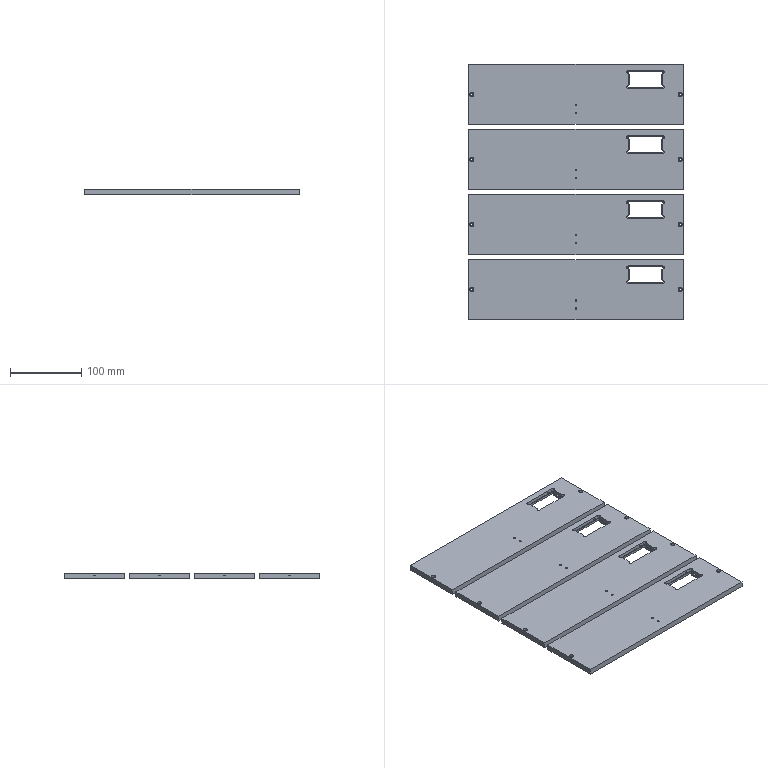Part | 4 solids | 188 faces | box 300 x 357 x 8 mm | volume 767552 mm3 | cylinder 96 | plane 84 | cone 8 | commonest cylinder face diameters 2.5 x32 4.2 x32 3.5 x16 6 x16